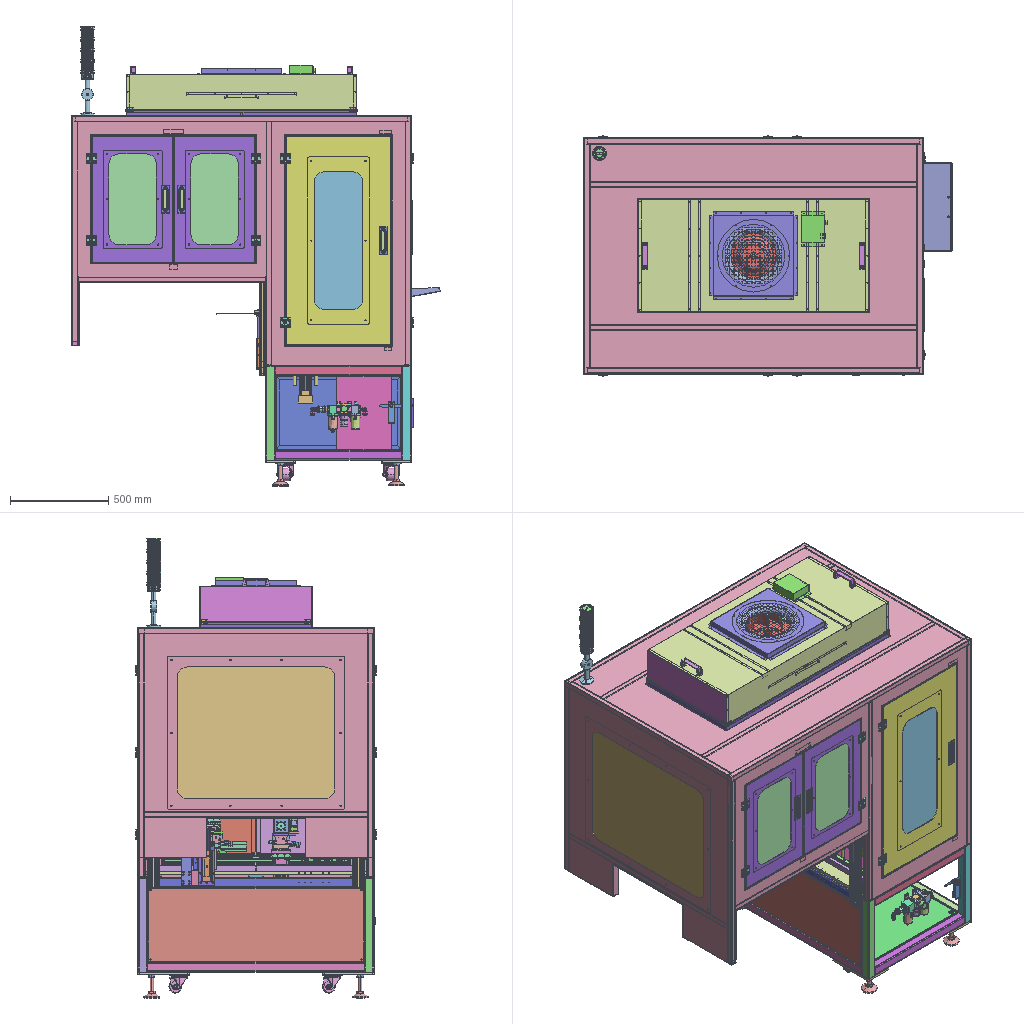Assembly | SolidWorks | 289 different items | 600 placed | box 1872 x 1223 x 2337 mm
Parts list (item | name | quantity | parent item | size | volume | features):
1 | (subassembly) | x1 | in 13 | 206.7 x 78.5 x 62 mm | 306344 mm3 | -
2 | (subassembly) | x1 | in 1 | 184.2 x 78.5 x 62 mm | 299098 mm3 | -
3 | (subassembly) | x1 | in 4 | 25 x 39 x 62 mm | 38108 mm3 | -
4 | (subassembly) | x1 | in 5 | 25 x 39 x 62 mm | 38108 mm3 | -
5 | (subassembly) | x1 | in 6 | 25 x 39 x 62 mm | 38108 mm3 | -
6 | (subassembly) | x1 | in 2 | 184.2 x 78.5 x 62 mm | 299098 mm3 | -
7 | (subassembly) | x1 | in 3 | 25 x 39 x 62 mm | 38108 mm3 | -
8 | (subassembly) | x1 | in 9 | 1174 x 574 x 303.9 mm | 75861290 mm3 | -
9 | (subassembly) | x1 | - | - | - | features InContextFeatHolder 8, CompositeCurve 1
10 | (subassembly) | x1 | in 12 | 740 x 1200 x 627 mm | 11363553 mm3 | features InContextFeatHolder 2
11 | (subassembly) | x1 | in 13 | 74.6 x 107 x 490 mm | 263242 mm3 | -
12 | (subassembly) | x1 | in 9 | - | 46022542 mm3 | features InContextFeatHolder 11, CompositeCurve 1
13 | (subassembly) | x1 | - | - | - | features InContextFeatHolder 122, ReferencePattern 9, AEMSimFeature 1, LocalLPattern 1
14 | (subassembly) | x1 | - | - | 2657898 mm3 | features InContextFeatHolder 6
15 | (subassembly) | x1 | in 13 | 960 x 40 x 48 mm | 597195 mm3 | -
16 | (subassembly) | x2 | in 13 | 570.077 x 115 x 65.1 mm | 63458 mm3 | features AEMSimFeature 1
17 | (subassembly) | x3 | in 13 | 380 x 48 x 106.85 mm | 542226 mm3 | -
18 | (subassembly) | x1 | in 27 | 150 x 20.749 x 140 mm | 48945 mm3 | -
19 | (subassembly) | x2 | in 13 | 60 x 10 x 20 mm | 6249 mm3 | -
20 | (subassembly) | x1 | in 13 | 80 x 32 x 65 mm | 107710 mm3 | features AEMSimFeature 1
21 | (subassembly) | x1 | in 13 | 97.6 x 32 x 65 mm | 120798 mm3 | features AEMSimFeature 1
22 | (subassembly) | x1 | in 31 | 62 x 9.5 x 27.6 mm | 10978 mm3 | -
23 | (subassembly) | x2 | in 13 | 175.3 x 32 x 65 mm | 205284 mm3 | features AEMSimFeature 1
24 | (subassembly) | x1 | in 13 | - | 4425715 mm3 | -
25 | (subassembly) | x2 | in 13 | 342 x 153.7 x 73.7 mm | 1636225 mm3 | -
26 | (subassembly) | x2 | in 24 | 88.4 x 8 x 103.5 mm | 9214 mm3 | -
27 | (subassembly) | x1 | in 9 | - | 566898 mm3 | -
28 | (subassembly) | x1 | in 14 | 204 x 189.5 x 238.5 mm | 703378 mm3 | -
29 | (subassembly) | x16 | in 12 | 50 x 11.3 x 50 mm | 15084 mm3 | -
30 | (subassembly) | x1 | in 22 | 62 x 9.5 x 27.6 mm | 10978 mm3 | -
31 | (subassembly) | x1 | in 7 | 25 x 39 x 62 mm | 38108 mm3 | -
32 | (subassembly) | x1 | in 27 | 244 x 14 x 167 mm | 40876 mm3 | -
33 | (subassembly) | x1 | in 9 | 167.4 x 157.9 x 105 mm | 781084 mm3 | features AEMSimFeature 1
34 | (subassembly) | x4 | in 10 | 185 x 80 x 80 mm | 147831 mm3 | -
35 | (subassembly) | x1 | in 13 | 179 x 58 x 20 mm | 151640 mm3 | features AEMSimFeature 1
36 | - | x2 | in 1 | 20 x 10 x 27.5 mm | 2836 mm3 | features BaseBody 1
37 | - | x2 | in 13 | 84 x 700 x 12 mm | 143164 mm3 | features HoleWzd 3, Fillet 1, FlatPattern 1, SMBaseFlange 1, SheetMetal 1
38 | - | x1 | in 13 | 70 x 25 x 57 mm | 49488 mm3 | features HoleWzd 2, Chamfer 1, Extrusion 1, ICE 1
39 | - | x4 | in 13 | 65 x 11 x 12 mm | 4036 mm3 | features ICE 5, Chamfer 4, Fillet 2, Extrusion 1, HoleWzd 1
40 | - | x1 | in 13 | 78 x 80 x 108.5 mm | 46050 mm3 | features HoleWzd 2, Fillet 1, FlatPattern 1, SMBaseFlange 1, SheetMetal 1
41 | - | x1 | in 13 | 120 x 20 x 10 mm | 22814 mm3 | features HoleWzd 2, ICE 2, Chamfer 1, Extrusion 1, LPattern 1
42 | - | x1 | in 13 | 80 x 15 x 180 mm | 211462 mm3 | features HoleWzd 3, Chamfer 1, Extrusion 1
43 | - | x1 | in 13 | 60 x 10 x 50 mm | 26983 mm3 | features HoleWzd 3, Chamfer 1, Extrusion 1, ICE 1
44 | - | x2 | in 13 | 50 x 8 x 56 mm | 20280 mm3 | features HoleWzd 8, Chamfer 2, Extrusion 1
45 | - | x1 | in 13 | 46.5 x 10 x 50 mm | 20990 mm3 | features HoleWzd 2, Chamfer 1, Extrusion 1
46 | - | x1 | in 13 | 25 x 10 x 110 mm | 24285 mm3 | features HoleWzd 3, Chamfer 1, Extrusion 1, ICE 1
47 | - | x1 | in 30 | 62 x 27.6 x 9.5 mm | 10978 mm3 | features BaseBody 1
48 | - | x1 | in 13 | 143 x 40 x 32 mm | 20017 mm3 | features HoleWzd 2, Fillet 1, FlatPattern 1, SMBaseFlange 1, SheetMetal 1
49 | - | x1 | in 13 | 233 x 40 x 32 mm | 34041 mm3 | features HoleWzd 2, ICE 2, Fillet 1, FlatPattern 1, SMBaseFlange 1, SheetMetal 1
50 | - | x1 | in 13 | 200 x 10 x 50 mm | 97100 mm3 | features HoleWzd 5, Chamfer 1, Extrusion 1
51 | - | x1 | in 13 | 50 x 10 x 240 mm | 114088 mm3 | features HoleWzd 2, Chamfer 1, Extrusion 1
52 | - | x1 | in 13 | 60 x 35 x 25.5 mm | 8094 mm3 | features HoleWzd 2, Fillet 1, FlatPattern 1, SMBaseFlange 1, SheetMetal 1
53 | - | x1 | in 13 | 80 x 40 x 75 mm | 17875 mm3 | features HoleWzd 2, Fillet 1, FlatPattern 1, SMBaseFlange 1, SheetMetal 1
54 | - | x1 | in 13 | 100 x 30 x 53 mm | 13622 mm3 | features HoleWzd 2, Fillet 1, FlatPattern 1, ICE 1, SMBaseFlange 1, SheetMetal 1
55 | - | x1 | in 13 | 70 x 50 x 75 mm | 19314 mm3 | features Fillet 2, HoleWzd 2, FlatPattern 1, ICE 1, SMBaseFlange 1, SheetMetal 1
56 | - | x2 | in 13 | 50 x 65 x 50.5 mm | 18737 mm3 | features HoleWzd 2, Fillet 1, FlatPattern 1, ICE 1, SMBaseFlange 1, SheetMetal 1
57 | - | x1 | in 13 | 70 x 50 x 75 mm | 19314 mm3 | features Fillet 2, HoleWzd 2, FlatPattern 1, ICE 1, SMBaseFlange 1, SheetMetal 1
58 | - | x1 | in 18 | 7.55 x 3.6 x 5.25 mm | 54.106 mm3 | features BaseBody 5
59 | - | x1 | in 13 | 170 x 10 x 75 mm | 122534 mm3 | features Chamfer 1, Cut 1, Extrusion 1
60 | - | x1 | in 13 | 67 x 70.75 x 50 mm | 14918 mm3 | features ICE 4, EdgeFlange 2, FlatPattern 2, HoleWzd 2, SMBaseFlange 2, SheetMetal 2, Fillet 1
61 | - | x1 | in 13 | 90 x 5 x 60 mm | 26435 mm3 | features Chamfer 1, Cut 1, Extrusion 1
62 | - | x1 | in 13 | 67 x 90.75 x 50 mm | 17594 mm3 | features ICE 5, EdgeFlange 2, Fillet 2, FlatPattern 2, HoleWzd 2, SMBaseFlange 2, SheetMetal 2, MirrorSolid 1
63 | - | x1 | in 13 | 27 x 70 x 27 mm | 8082 mm3 | features HoleWzd 2, EdgeFlange 1, Fillet 1, FlatPattern 1, ICE 1, SMBaseFlange 1, SheetMetal 1
64 | - | x1 | - | 27 x 70 x 27 mm | 8082 mm3 | features HoleWzd 2, ICE 2, EdgeFlange 1, Fillet 1, FlatPattern 1, MirrorSolid 1, SMBaseFlange 1, SheetMetal 1
65 | - | x2 | in 13 | 100 x 30 x 60 mm | 72680 mm3 | features HoleWzd 2, Chamfer 1, Extrusion 1, ICE 1
66 | - | x1 | in 13 | 65 x 46.5 x 55 mm | 13185 mm3 | features HoleWzd 4, ICE 3, EdgeFlange 2, FlatPattern 2, SMBaseFlange 2, SheetMetal 2, Cut 1, Fillet 1
67 | - | x1 | in 13 | 65 x 31.5 x 55 mm | 13652 mm3 | features HoleWzd 4, EdgeFlange 2, FlatPattern 2, ICE 2, SMBaseFlange 2, SheetMetal 2, Fillet 1
68 | - | x1 | in 13 | 50 x 3 x 45 mm | 6177 mm3 | features Chamfer 1, Extrusion 1, HoleWzd 1
69 | - | x1 | in 18 | 5.1 x 2 x 11 mm | 74.432 mm3 | features BaseBody 1
70 | - | x2 | in 13 | 30 x 22 x 30 mm | 5974 mm3 | features HoleWzd 3, ICE 2, Chamfer 1, Extrusion 1
71 | - | x2 | in 13 | 25 x 30 x 60 mm | 17122 mm3 | features HoleWzd 3, ICE 2, Chamfer 1, Extrusion 1
72 | - | x2 | in 13 | 8 x 75 x 8 mm | 3681 mm3 | features Extrusion 1, HoleWzd 1
73 | - | x2 | in 13 | 10 x 25 x 20 mm | 4403 mm3 | features HoleWzd 3, Chamfer 1, Extrusion 1, ICE 1
74 | - | x2 | in 13 | 12 x 15 x 20 mm | 2799 mm3 | features Chamfer 1, Extrusion 1, HoleWzd 1
75 | - | x2 | in 14 | 30 x 60 x 560 mm | 279456 mm3 | features HoleWzd 1, WeldMemberFeat 1, WeldmentFeature 1
76 | - | x1 | in 14 | 30 x 60 x 980 mm | 490298 mm3 | features WeldMemberFeat 1, WeldmentFeature 1
77 | - | x2 | in 14 | 63 x 60 x 63 mm | 21324 mm3 | features HoleWzd 2, Fillet 1, FlatPattern 1, ICE 1, SMBaseFlange 1, SheetMetal 1
78 | - | x1 | - | 30 x 60 x 300 mm | 150091 mm3 | features WeldMemberFeat 1, WeldmentFeature 1
79 | - | x1 | - | 60 x 60 x 60 mm | 62996 mm3 | features HoleWzd 2, Chamfer 1, Extrusion 1, ICE 1
80 | - | x1 | in 18 | 28.83 x 2.1 x 4.91 mm | 297.266 mm3 | features BaseBody 1
81 | - | x2 | in 14 | 120 x 10 x 120 mm | 98760 mm3 | features Chamfer 1, Extrusion 1, Fillet 1, HoleWzd 1, ICE 1
82 | - | x1 | in 14 | 230 x 10 x 205 mm | 459180 mm3 | features HoleWzd 3, Chamfer 1, Extrusion 1
83 | - | x2 | in 14 | 120 x 10 x 60 mm | 66873 mm3 | features HoleWzd 3, Chamfer 1, Extrusion 1
84 | - | x2 | in 14 | 90 x 10 x 60 mm | 36102 mm3 | features HoleWzd 2, Chamfer 1, Extrusion 1, ICE 1
85 | - | x4 | in 12 | 414.5 x 646 x 20 mm | 455877 mm3 | features HoleWzd 3, ICE 3, EdgeFlange 2, Cut 1, FlatPattern 1, LPattern 1, SMBaseFlange 1, SheetMetal 1
86 | - | x4 | in 12 | 300 x 500 x 5 mm | 748723 mm3 | features Extrusion 1, Fillet 1, HoleWzd 1
87 | - | x1 | in 27 | 235 x 5 x 143 mm | 168025 mm3 | features BaseBody 1
88 | - | x1 | in 33 | 37.5 x 37.5 x 40.6 mm | 27619 mm3 | features BaseBody 1
89 | - | x1 | in 15 | 48 x 34.5 x 84 mm | 102162 mm3 | features BaseBody 5
90 | - | x1 | in 15 | 48 x 34.5 x 84 mm | 102161 mm3 | features BaseBody 5
91 | - | x1 | in 18 | 16 x 8.47 x 16.6 mm | 886.614 mm3 | features BaseBody 1
92 | - | x1 | in 15 | 23 x 22 x 960 mm | 392872 mm3 | features BaseBody 1
93 | - | x1 | in 13 | 32 x 55 x 30 mm | 32416 mm3 | features ICE 2, Extrusion 1, HoleWzd 1, LPattern 1
94 | - | x1 | in 13 | - | - | features BaseBody 3, RefSurface 1
95 | - | x8 | in 9 | 30 x 91 x 31 mm | 76497 mm3 | features BaseBody 2
96 | - | x8 | in 9 | 48.4 x 47.5 x 16.6 mm | 8438 mm3 | features BaseBody 7, MoveCopyBody 1
97 | - | x1 | in 9 | 35.5 x 35.5 x 68.5 mm | 34572 mm3 | features BaseBody 2
98 | - | x1 | in 18 | 47.6 x 49.1 x 3.35 mm | 7804 mm3 | features BaseBody 1
99 | - | x3 | in 13 | 174.25 x 62 x 80 mm | 431030 mm3 | features HoleWzd 2, Sweep 1
100 | - | x4 | in 16 | 32 x 7 x 58 mm | 8749 mm3 | features BaseBody 1
101 | - | x2 | in 16 | 58.5 x 35 x 65 mm | 23683 mm3 | features BaseBody 1
102 | - | x1 | in 18 | 14.571 x 11.26 x 19.95 mm | 1672 mm3 | features BaseBody 1
103 | - | x2 | in 16 | 58.5 x 35 x 65 mm | 22276 mm3 | features BaseBody 1
104 | - | x30 | in 16 | - | - | features BaseBody 1
105 | - | x3 | in 17 | 94 x 36 x 82.5 mm | 126431 mm3 | features BaseBody 1
106 | - | x3 | in 17 | 62 x 47 x 370 mm | 387917 mm3 | features BaseBody 1
107 | - | x3 | in 17 | 42 x 42 x 11 mm | 10971 mm3 | features BaseBody 1
108 | - | x3 | in 17 | 8 x 5 x 300 mm | 5669 mm3 | features BaseBody 1
109 | - | x6 | in 17 | 27.675 x 17 x 32.6 mm | 3746 mm3 | features BaseBody 1
110 | - | x3 | in 17 | 27.675 x 17 x 32.6 mm | 3746 mm3 | features BaseBody 1
111 | - | x8 | in 13 | 34 x 48 x 70 mm | 33372 mm3 | features BaseBody 1
112 | - | x2 | in 13 | 24 x 32 x 21 mm | 5040 mm3 | features HoleWzd 2, ICE 2, CirPattern 1, Extrusion 1
113 | - | x1 | in 18 | 15.807 x 7.64 x 18.249 mm | 686.202 mm3 | features BaseBody 1
114 | - | x8 | in 12 | - | - | features BaseBody 6, RefSurface 2
115 | - | x8 | in 12 | 13 x 13 x 37 mm | 2260 mm3 | features ICE 2, Extrusion 1
116 | - | x2 | in 19 | 20 x 8 x 28.9 mm | 3330 mm3 | features BaseBody 5
117 | - | x2 | in 19 | 9 x 6.5 x 60 mm | 2919 mm3 | features BaseBody 1, ICE 1
118 | - | x3 | in 12 | 120 x 110 x 37 mm | 69257 mm3 | features ICE 6, Fillet 4, Chamfer 1, Extrusion 1, MirrorPattern 1
119 | - | x1 | in 18 | 150 x 1.6 x 140 mm | 32858 mm3 | features BaseBody 1
120 | - | x1 | in 20 | 8 x 8 x 20 mm | 908.839 mm3 | features BaseBody 1
121 | - | x1 | in 21 | 8 x 8 x 20 mm | 908.839 mm3 | features BaseBody 1
122 | - | x1 | in 20 | 12 x 13.856 x 4 mm | 340.073 mm3 | features BaseBody 1
123 | - | x1 | in 21 | 12 x 13.856 x 4 mm | 340.073 mm3 | features BaseBody 1
124 | - | x1 | in 18 | 18.3 x 13.55 x 20.425 mm | 1911 mm3 | features BaseBody 1
125 | - | x1 | in 20 | 13 x 10 x 18.5 mm | 2290 mm3 | features BaseBody 1
126 | - | x1 | in 21 | 13 x 10 x 18.5 mm | 2290 mm3 | features BaseBody 1
127 | - | x1 | in 20 | 16 x 31 x 9.5 mm | 4071 mm3 | features BaseBody 1
128 | - | x1 | in 21 | 16 x 31 x 9.5 mm | 4071 mm3 | features BaseBody 1
129 | - | x2 | in 23 | 12 x 13.856 x 4 mm | 339.344 mm3 | features BaseBody 1
130 | - | x2 | in 23 | 16 x 31 x 9.5 mm | 4071 mm3 | features BaseBody 1
131 | - | x2 | in 23 | 15 x 10 x 20.5 mm | 2936 mm3 | features BaseBody 1
132 | - | x1 | in 20 | 47 x 26.5 x 70 mm | 54767 mm3 | features BaseBody 1
133 | - | x1 | in 20 | 50 x 29 x 79 mm | 45333 mm3 | features BaseBody 1
134 | - | x1 | in 21 | 47 x 26.5 x 82 mm | 60945 mm3 | features BaseBody 1
135 | - | x1 | in 18 | 12.55 x 30.81 x 17.2 mm | 2595 mm3 | features BaseBody 1
136 | - | x1 | in 21 | 50 x 29 x 91 mm | 51453 mm3 | features BaseBody 1
137 | - | x2 | in 23 | 47 x 26.5 x 148 mm | 111370 mm3 | features BaseBody 1
138 | - | x2 | in 23 | 50 x 29 x 157 mm | 83904 mm3 | features BaseBody 1
139 | - | x4 | in 23 | 4 x 4.5 x 32 mm | 371.041 mm3 | features BaseBody 1
140 | - | x2 | in 21 | 4 x 4.6 x 32 mm | 394.901 mm3 | features BaseBody 1
141 | - | x2 | in 9 | 39.315 x 43.5 x 21 mm | 8972 mm3 | features BaseBody 1
142 | - | x1 | in 1 | 26 x 14.6 x 15 mm | 1573 mm3 | features BaseBody 1
143 | - | x1 | in 9 | 70.234 x 70.234 x 455.4 mm | 394437 mm3 | features BaseBody 7, ICE 3, HoleWzd 2, MoveCopyBody 2, Fillet 1, Stock 1
144 | - | x2 | in 23 | 40.8 x 8 x 8 mm | 1922 mm3 | features BaseBody 1
145 | - | x1 | in 24 | 111.5 x 65 x 930 mm | 2439001 mm3 | features BaseBody 1
146 | - | x2 | in 25 | 66 x 153.7 x 73.7 mm | 524203 mm3 | features BaseBody 1
147 | - | x1 | in 18 | 7.5 x 10.5 x 3.3 mm | 105.725 mm3 | features BaseBody 1
148 | - | x2 | in 24 | 110 x 49 x 100 mm | 206200 mm3 | features BaseBody 1
149 | - | x1 | in 24 | 82 x 17.089 x 949 mm | 309530 mm3 | features BaseBody 1
150 | - | x2 | in 24 | 920 x 12.53 x 15 mm | 149023 mm3 | features BaseBody 1
151 | - | x8 | in 24 | 40.3 x 19.5 x 34 mm | 21226 mm3 | features BaseBody 1
152 | - | x2 | in 9 | 120 x 120 x 25 mm | 99576 mm3 | features Boss 5, Fillet 2, CirPattern 1, Cut 1, Extrusion 1, HoleWzd 1
153 | - | x2 | in 25 | 60 x 171.6 x 72.85 mm | 479622 mm3 | features BaseBody 1
154 | - | x1 | - | 51 x 26 x 73 mm | 95067 mm3 | features Extrusion 1, Fillet 1, HoleWzd 1, ICE 1
155 | - | x2 | in 13 | 5 x 15 x 5 mm | 252.815 mm3 | features Chamfer 1, Extrusion 1, HoleWzd 1
156 | - | x2 | in 33 | 16.2 x 43 x 13.5 mm | 6701 mm3 | features BaseBody 1
157 | - | x2 | in 33 | 7.5 x 43 x 30 mm | 4813 mm3 | features BaseBody 1
158 | - | x12 | in 27 | 6 x 10 x 6 mm | 109.62 mm3 | features BaseBody 1
159 | - | x2 | in 33 | 20 x 85 x 28 mm | 22186 mm3 | features BaseBody 1
160 | - | x2 | in 26 | 31 x 8 x 25 mm | 3494 mm3 | features BaseBody 1
161 | - | x2 | in 26 | 76.4 x 83.5 x 7 mm | 5719 mm3 | features BaseBody 1
162 | - | x2 | in 24 | 50 x 53.1 x 100 mm | 115973 mm3 | features BaseBody 1
163 | - | x2 | in 24 | 18 x 18 x 1.5 mm | 454.137 mm3 | features BaseBody 1
164 | - | x1 | in 24 | 50 x 10.1 x 120 mm | 50542 mm3 | features BaseBody 1
165 | - | x4 | in 24 | 50 x 10.1 x 200 mm | 84250 mm3 | features BaseBody 1
166 | - | x2 | in 24 | 18 x 14 x 4 mm | 787.982 mm3 | features BaseBody 1
167 | - | x2 | in 24 | 45 x 15 x 17 mm | 8178 mm3 | features BaseBody 1
168 | - | x2 | in 24 | 56.42 x 14.8 x 12 mm | 6251 mm3 | features BaseBody 1
169 | - | x1 | in 27 | 265 x 193 x 0.32 mm | 7343 mm3 | features BaseBody 1
170 | - | x4 | in 24 | 17 x 17 x 10 mm | 1547 mm3 | features BaseBody 1
171 | - | x1 | in 13 | 158.45 x 26.5 x 60 mm | 118461 mm3 | features BaseBody 3
172 | - | x2 | in 8 | 19.9 x 568.8 x 179.4 mm | 76913 mm3 | features BaseBody 1
173 | - | x2 | in 8 | 58.8 x 560 x 25 mm | 35807 mm3 | features BaseBody 1
174 | - | x1 | in 28 | 11 x 38.188 x 38.188 mm | 8381 mm3 | features BaseBody 1
175 | - | x1 | - | 27 x 11 x 89 mm | 6132 mm3 | features ICE 3, Chamfer 2, Fillet 2, ExtruThin 1
176 | - | x1 | in 8 | 29.6 x 34.2 x 22.3 mm | 11730 mm3 | features BaseBody 1
177 | - | x2 | in 8 | 136.5 x 40 x 26 mm | 27538 mm3 | features BaseBody 1
178 | - | x1 | - | 27 x 11 x 89 mm | 6132 mm3 | features Fillet 2, ICE 2, Chamfer 1, ExtruThin 1
179 | - | x1 | in 28 | 203 x 228 x 6 mm | 252836 mm3 | features BaseBody 1
180 | - | x2 | in 32 | 10 x 2 x 21 mm | 420 mm3 | features BaseBody 1
181 | - | x1 | in 8 | 178.6 x 44.9 x 114.8 mm | 25020 mm3 | features BaseBody 1
182 | - | x1 | in 28 | 110 x 40 x 10 mm | 12474 mm3 | features BaseBody 1
183 | - | x1 | in 9 | 270 x 35 x 167 mm | 892435 mm3 | features Fillet 3, ICE 3, Extrusion 1, HoleWzd 1
184 | - | x11 | in 13 | 2 x 34 x 2 mm | 106.814 mm3 | features Extrusion 1
185 | - | x1 | in 8 | 40 x 20 x 40 mm | 945.968 mm3 | features BaseBody 1
186 | - | x1 | in 8 | 170 x 568.8 x 20 mm | 69593 mm3 | features BaseBody 1
187 | - | x1 | in 28 | 58 x 13.5 x 49 mm | 21022 mm3 | features BaseBody 1
188 | - | x1 | in 28 | 203 x 133.5 x 222.9 mm | 123342 mm3 | features BaseBody 1
189 | - | x1 | in 8 | 1169 x 570 x 180 mm | 606575 mm3 | features BaseBody 1
190 | - | x1 | in 8 | 560 x 568.8 x 17.4 mm | 168286 mm3 | features BaseBody 1
191 | - | x1 | in 27 | 270.8 x 5.7 x 198.8 mm | 17493 mm3 | features BaseBody 1
192 | - | x1 | in 28 | 13 x 35 x 35 mm | 3307 mm3 | features BaseBody 1
193 | - | x1 | in 28 | 204 x 141.5 x 3.5 mm | 90063 mm3 | features BaseBody 1
194 | - | x4 | in 28 | 19.046 x 16 x 19.046 mm | 2136 mm3 | features BaseBody 1
195 | - | x4 | in 11 | 19.513 x 16 x 19.513 mm | 2386 mm3 | features BaseBody 1
196 | - | x1 | in 8 | 30 x 30 x 37 mm | 14720 mm3 | features BaseBody 1
197 | - | x3 | in 11 | 5 x 8 x 8 mm | 228.346 mm3 | features BaseBody 1
198 | - | x2 | in 8 | 40 x 20 x 40 mm | 945.968 mm3 | features BaseBody 1
199 | - | x1 | in 8 | 40 x 20 x 40 mm | 945.968 mm3 | features BaseBody 1
200 | - | x1 | in 13 | 36 x 28.1 x 36 mm | 26906 mm3 | features Extrusion 1, ICE 1
201 | - | x1 | in 11 | 347 x 40 x 40 mm | 65836 mm3 | features BaseBody 1, ICE 1
202 | - | x1 | in 27 | 35.585 x 17.1 x 141.528 mm | 13223 mm3 | features BaseBody 1
203 | - | x1 | - | 8 x 8 x 20 mm | 605.018 mm3 | features Chamfer 1, Extrusion 1, ICE 1, MirrorPattern 1
204 | - | x1 | in 28 | 222.8 x 84 x 5 mm | 93378 mm3 | features BaseBody 1
205 | - | x1 | in 28 | 204 x 141.5 x 3.5 mm | 90078 mm3 | features BaseBody 1
206 | - | x2 | in 9 | 117.5 x 5.2 x 117.5 mm | 4285 mm3 | features Boss 1, CompositeCurve 1, MirrorPattern 1, Revolution 1, Sweep 1
207 | - | x1 | in 8 | 1170 x 79 x 570 mm | 72868307 mm3 | features BaseBody 6
208 | - | x1 | in 27 | 272.622 x 33.34 x 200.622 mm | 144122 mm3 | features BaseBody 1
209 | - | x1 | in 27 | 256 x 1 x 184 mm | 42983 mm3 | features BaseBody 1
210 | - | x1 | in 32 | 244 x 12 x 167 mm | 40036 mm3 | features BaseBody 1
211 | - | x1 | in 8 | 395 x 93 x 395 mm | 708479 mm3 | features BaseBody 1
212 | - | x2 | in 25 | 200 x 53 x 53 mm | 525174 mm3 | features BaseBody 1
213 | - | x1 | in 8 | 370 x 30.2 x 370 mm | 96881 mm3 | features BaseBody 1
214 | - | x1 | in 8 | 154 x 120 x 154 mm | 897140 mm3 | features BaseBody 2
215 | - | x1 | in 8 | 448.8 x 29.9 x 448.6 mm | 111813 mm3 | features BaseBody 1
216 | - | x2 | in 24 | 22 x 37.5 x 8 mm | 1327 mm3 | features BaseBody 1
217 | - | x1 | in 27 | 152.5 x 244.9 x 2.34 mm | 82614 mm3 | features BaseBody 1
218 | - | x1 | in 31 | 54 x 39 x 15.5 mm | 27130 mm3 | features BaseBody 1
219 | - | x1 | in 33 | 53 x 53.5 x 53 mm | 128683 mm3 | features BaseBody 1
220 | - | x1 | in 33 | 46.4 x 74.3 x 53.2 mm | 114599 mm3 | features BaseBody 1
221 | - | x1 | in 33 | 19.5 x 11.1 x 8 mm | 1041 mm3 | features BaseBody 1
222 | - | x1 | in 33 | 53 x 70.1 x 53 mm | 131657 mm3 | features BaseBody 1
223 | - | x2 | in 24 | 110 x 15 x 92 mm | 55640 mm3 | features BaseBody 1
224 | - | x1 | in 33 | 46.4 x 74.3 x 53.2 mm | 114523 mm3 | features BaseBody 1
225 | - | x1 | in 33 | 53 x 52 x 53 mm | 114626 mm3 | features BaseBody 1
226 | - | x1 | in 33 | 53 x 65 x 53 mm | 80542 mm3 | features BaseBody 1
227 | - | x4 | in 34 | 185 x 80 x 80 mm | 139335 mm3 | features BaseBody 1
228 | - | x4 | in 34 | 16 x 34.641 x 30 mm | 8496 mm3 | features BaseBody 1
229 | - | x4 | in 10 | 102.5 x 95 x 100 mm | 269431 mm3 | features BaseBody 4
230 | - | x32 | in 29 | 31 x 11.3 x 50 mm | 6837 mm3 | features BaseBody 1
231 | - | x16 | in 29 | 6 x 6 x 50 mm | 1409 mm3 | features MoveCopyBody 5, BaseBody 1
232 | - | x1 | in 35 | 20 x 58 x 169 mm | 126513 mm3 | features BaseBody 1
233 | - | x1 | in 35 | 18 x 56 x 154 mm | 25127 mm3 | features BaseBody 1
234 | - | x1 | in 33 | 9.728 x 9.728 x 6.2 mm | 395.486 mm3 | features BaseBody 1
235 | - | x1 | in 6 | 160.8 x 46.8 x 78.5 mm | 260990 mm3 | features BaseBody 1
236 | - | x1 | - | 33 x 37.5 x 33 mm | 22047 mm3 | features Chamfer 1, Extrusion 1, RevCut 1
237 | - | x1 | - | 40 x 40 x 39 mm | 38929 mm3 | features Extrusion 1, ICE 1
238 | - | x2 | in 9 | 148.5 x 148.5 x 29 mm | 366901 mm3 | features HoleWzd 2, ICE 2, Extrusion 1, LPattern 1
239 | - | x3 | in 13 | 117.111 x 104.2 x 58.651 mm | 144018 mm3 | features BaseBody 2
240 | - | x4 | in 24 | 13.7 x 28.4 x 26 mm | 1939 mm3 | features BaseBody 1
241 | - | x1 | in 10 | 50 x 50 x 480 mm | 259595 mm3 | features WeldMemberFeat 1, WeldmentFeature 1
242 | - | x1 | in 10 | 50 x 50 x 480 mm | 259595 mm3 | features WeldMemberFeat 1, WeldmentFeature 1
243 | - | x1 | in 10 | 50 x 50 x 640 mm | 345950 mm3 | features HoleWzd 1, WeldMemberFeat 1, WeldmentFeature 1
244 | - | x1 | in 10 | 50 x 50 x 640 mm | 346127 mm3 | features WeldMemberFeat 1, WeldmentFeature 1
245 | - | x1 | in 11 | 170 x 73 x 8 mm | 75730 mm3 | features BaseBody 1
246 | - | x1 | in 10 | 50 x 50 x 1100 mm | 594670 mm3 | features HoleWzd 1, WeldMemberFeat 1, WeldmentFeature 1
247 | - | x1 | in 10 | 50 x 50 x 640 mm | 346127 mm3 | features WeldMemberFeat 1, WeldmentFeature 1
248 | - | x1 | in 10 | 50 x 50 x 640 mm | 345950 mm3 | features HoleWzd 1, WeldMemberFeat 1, WeldmentFeature 1
249 | - | x1 | in 10 | 50 x 50 x 480 mm | 259595 mm3 | features WeldMemberFeat 1, WeldmentFeature 1
250 | - | x1 | in 10 | 50 x 50 x 1100 mm | 594018 mm3 | features HoleWzd 4, WeldMemberFeat 1, WeldmentFeature 1
251 | - | x1 | in 10 | 50 x 50 x 1100 mm | 594905 mm3 | features WeldMemberFeat 1, WeldmentFeature 1
252 | - | x1 | in 10 | 50 x 50 x 1100 mm | 594905 mm3 | features WeldMemberFeat 1, WeldmentFeature 1
253 | - | x1 | in 10 | 50 x 50 x 480 mm | 259595 mm3 | features WeldMemberFeat 1, WeldmentFeature 1
254 | - | x4 | in 10 | 150 x 12 x 260 mm | 462019 mm3 | features HoleWzd 2, Extrusion 1, Fillet 1
255 | - | x4 | in 10 | 44 x 3 x 44 mm | 5785 mm3 | features Extrusion 1, Fillet 1
256 | - | x1 | in 11 | 73.2 x 90 x 163.5 mm | 60174 mm3 | features BaseBody 1
257 | - | x1 | in 10 | 20 x 1100 x 640 mm | 1523319 mm3 | features Cut 1, EdgeFlange 1, FlatPattern 1, SMBaseFlange 1, SheetMetal 1
258 | - | x4 | in 10 | 40 x 5 x 40 mm | 3902 mm3 | features Extrusion 1, HoleWzd 1
259 | - | x9 | in 10 | 80 x 15 x 80 mm | 95133 mm3 | features Extrusion 1, Fillet 1, HoleWzd 1
260 | - | x1 | in 10 | 50 x 50 x 1100 mm | 594905 mm3 | features WeldMemberFeat 1, WeldmentFeature 1
261 | - | x3 | in 10 | 45 x 10 x 40 mm | 11000 mm3 | features Extrusion 1, ICE 1
262 | - | x1 | in 12 | 560 x 402 x 22 mm | 485747 mm3 | features MoveCopyBody 4, Stock 4, EdgeFlange 3, ICE 2, Cut 1, FlatPattern 1, LPattern 1, SMBaseFlange 1, SheetMetal 1
263 | - | x1 | in 12 | 376 x 1096 x 20 mm | 1022665 mm3 | features EdgeFlange 2, FlatPattern 1, HoleWzd 1, SMBaseFlange 1, SheetMetal 1
264 | - | x1 | in 12 | 636 x 390 x 20 mm | 609250 mm3 | features EdgeFlange 2, MoveCopyBody 2, Stock 2, FlatPattern 1, ICE 1, SMBaseFlange 1, SheetMetal 1
265 | - | x1 | in 12 | 1270 x 1200 x 1725 mm | 14201565 mm3 | features EdgeFlange 19, ICE 17, FlatPattern 11, HoleWzd 11, Fillet 7, SMBaseFlange 7, SheetMetal 7, MirrorSolid 2, 3DProfileFeature 1, Cut 1, MirrorPattern 1, WeldMemberFeat 1, WeldmentFeature 1
266 | - | x2 | in 12 | 315 x 850 x 5 mm | 1337473 mm3 | features Extrusion 1, Fillet 1, HoleWzd 1
267 | - | x1 | in 11 | 74 x 98 x 4.5 mm | 27198 mm3 | features BaseBody 1
268 | - | x2 | in 12 | 536 x 1066 x 20 mm | 1021642 mm3 | features ICE 4, HoleWzd 3, EdgeFlange 2, Cut 1, FlatPattern 1, LPattern 1, SMBaseFlange 1, SheetMetal 1
269 | - | x1 | in 12 | 497 x 1066 x 20 mm | 1161554 mm3 | features Cut 2, EdgeFlange 2, HoleWzd 2, ICE 2, LPattern 2, FlatPattern 1, SMBaseFlange 1, SheetMetal 1
270 | - | x1 | in 12 | 497 x 1066 x 48 mm | 1342726 mm3 | features Cut 6, EdgeFlange 4, HoleWzd 4, FlatPattern 2, SMBaseFlange 2, SheetMetal 2, ICE 1
271 | - | x1 | in 12 | 448 x 165 x 40 mm | 228606 mm3 | features ICE 4, EdgeFlange 3, HoleWzd 3, Fillet 1, FlatPattern 1, SMBaseFlange 1, SheetMetal 1
272 | - | x1 | in 12 | 40 x 41.5 x 80 mm | 9432 mm3 | features Fillet 1, FlatPattern 1, HoleWzd 1, SMBaseFlange 1, SheetMetal 1
273 | - | x1 | in 12 | 280 x 550 x 375 mm | 1500935 mm3 | features EdgeFlange 3, Cut 2, ICE 2, FlatPattern 1, SMBaseFlange 1, SheetMetal 1
274 | - | x1 | in 12 | 15 x 325 x 500 mm | 418730 mm3 | features EdgeFlange 2, FlatPattern 1, ICE 1, SMBaseFlange 1, SheetMetal 1
275 | - | x1 | in 12 | 900 x 780 x 5 mm | 3507647 mm3 | features Extrusion 1, Fillet 1, HoleWzd 1
276 | - | x1 | in 13 | 1120 x 15 x 700 mm | 9247441 mm3 | features HoleWzd 10, Cut 2, Chamfer 1, Extrusion 1, Fillet 1
277 | - | x1 | in 13 | 100 x 15 x 350 mm | 438251 mm3 | features HoleWzd 6, ICE 3, Chamfer 1, Extrusion 1
278 | - | x1 | in 11 | 74 x 98 x 4.5 mm | 24076 mm3 | features BaseBody 1
279 | - | x1 | in 13 | 20 x 300 x 160 mm | 940820 mm3 | features HoleWzd 5, Chamfer 1, Extrusion 1, ICE 1
280 | - | x1 | in 13 | 300 x 20 x 80 mm | 463875 mm3 | features HoleWzd 4, Chamfer 1, Extrusion 1, ICE 1
281 | - | x1 | in 13 | 120 x 10 x 200 mm | 194374 mm3 | features HoleWzd 6, Chamfer 2, Extrusion 1, Fillet 1, ICE 1
282 | - | x1 | in 13 | 210 x 10 x 90 mm | 139703 mm3 | features HoleWzd 4, Chamfer 2, Extrusion 1, Fillet 1, ICE 1
283 | - | x1 | in 13 | 260 x 10 x 90 mm | 149509 mm3 | features HoleWzd 7, Chamfer 1, Extrusion 1, ICE 1
284 | - | x1 | in 13 | 120 x 15 x 350 mm | 538843 mm3 | features HoleWzd 6, Cut 2, Chamfer 1, Extrusion 1, ICE 1
285 | - | x8 | in 13 | 16 x 250 x 16 mm | 49961 mm3 | features Extrusion 1, HoleWzd 1
286 | - | x2 | in 13 | 499 x 30 x 50 mm | 739765 mm3 | features HoleWzd 2, Chamfer 1, Extrusion 1
287 | - | x2 | in 13 | 100 x 25 x 55 mm | 120725 mm3 | features HoleWzd 4, Chamfer 1, Extrusion 1, ICE 1
288 | - | x2 | in 13 | 60 x 20 x 100 mm | 92174 mm3 | features HoleWzd 2, Chamfer 1, Extrusion 1, ICE 1
289 | - | x2 | in 25 | 90.5 x 53 x 53 mm | 107227 mm3 | features BaseBody 1
Mates (type | each side: item.copy, entity, surface, feature), first 260 of 652 lines:
In the top assembly
Coincident | 259.1 face plane Boss-Extrude 1 | 276.1 face plane Boss-Extrude 1
Width | 276.1 face plane Boss-Extrude 1 | 276.1 face plane Boss-Extrude 1 | 248.1 face plane Gb/6728-1986 Square Hollow Section 050 X 50 X 3(1) | 243.1 face plane Gb/6728-1986 Square Hollow Section 050 X 50 X 3(1)
Coincident | 250.1 face plane Gb/6728-1986 Square Hollow Section 050 X 50 X 3(1) | 276.1 face plane Boss-Extrude 1
Coincident | 250.1 face plane Gb/6728-1986 Square Hollow Section 050 X 50 X 3(1) | 75.1 face plane Aluminium Profile 30 X 60L X R2.5(1) | 3 times
In subassembly 13
Coincident | 276.2 face plane Boss-Extrude 1 | 286.1 face plane Boss-Extrude 1
Coincident | 277.1 face plane Boss-Extrude 1 | 288.1 face plane Boss-Extrude 1 | 2 times
Coincident | 285.1 face plane Boss-Extrude 1 | 285.2 face plane Boss-Extrude 1
Coincident | 277.1 face plane Boss-Extrude 1 | 287.1 face plane Boss-Extrude 1 | 2 times
Coincident | 280.1 face plane Cut-Extrude 1 | 285.1 face plane Boss-Extrude 1
DistanceDim | 286.1 face plane Boss-Extrude 1 | 276.2 face plane Boss-Extrude 1
Coincident | 285.3 face plane Boss-Extrude 1 | 285.4 face plane Boss-Extrude 1
Coincident | 284.1 face plane Boss-Extrude 1 | 288.2 face plane Boss-Extrude 1
Width | 279.1 face plane Boss-Extrude 1 | 279.1 face plane Boss-Extrude 1 | 284.1 face plane Boss-Extrude 1 | 284.1 face plane Boss-Extrude 1
Coincident | 279.1 face plane Cut-Extrude 1 | 285.4 face plane Boss-Extrude 1
Concentric | 288.1 face cylinder Cut-Extrude 1 | 289.1 face cylinder  Import 1
Coincident | 288.1 face plane Boss-Extrude 1 | 289.1 face plane  Import 1
Parallel | 288.1 face plane Boss-Extrude 1 | 289.1 face plane  Import 1
Concentric | 277.1 face cylinder Cut-Extrude 2 | 289.1 face cylinder  Import 1
Coincident | 276.2 face plane Boss-Extrude 1 | 37.1 face plane Base-Flange 1
Width | 37.1 face plane Base-Flange 1 | 37.1 face plane Base-Flange 1 | 276.2 face plane Boss-Extrude 1 | 276.2 face plane Boss-Extrude 1
Coincident | 276.2 face plane Boss-Extrude 1 | 145.1 face plane  Import 1
Width | 277.1 face plane Cut-Extrude 1 | 277.1 face plane Cut-Extrude 1 | 148.1 face plane  Import 1 | 148.1 face plane  Import 1
Width | 277.1 face plane Boss-Extrude 1 | 277.1 face plane Boss-Extrude 1 | 148.1 face plane  Import 1 | 148.1 face plane  Import 1
Width | 284.1 face plane Boss-Extrude 1 | 284.1 face plane Boss-Extrude 1 | 148.2 face plane  Import 1 | 148.2 face plane  Import 1
Width | 223.1 face plane  Import 2 | 223.2 face plane  Import 2 | 276.2 face plane Boss-Extrude 1 | 276.2 face plane Boss-Extrude 1
Coincident | 284.1 face plane Cut-Extrude 1 | 148.2 face plane  Import 1
Width | 284.1 face plane Cut-Extrude 1 | 284.1 face plane Cut-Extrude 1 | 148.2 face plane  Import 1 | 148.2 face plane  Import 1
Coincident | 277.1 face plane Cut-Extrude 1 | 148.1 face plane  Import 1
Width | 287.2 face plane Boss-Extrude 1 | 287.2 face plane Boss-Extrude 1 | 89.1 face plane  Import 4 | 89.1 face plane  Import 4 | 2 times
Coincident | 287.2 face plane Cut-Extrude 1 | 89.1 face plane  Import 4
Coincident | 287.1 face plane Cut-Extrude 1 | 90.1 face plane  Import 4
Width | 287.1 face plane Boss-Extrude 1 | 287.1 face plane Boss-Extrude 1 | 90.1 face plane  Import 4 | 90.1 face plane  Import 4 | 2 times
LimitDistanceDim | 289.1 face plane  Import 1 | 280.1 face plane Cut-Extrude 1
Coincident | 276.2 face plane Boss-Extrude 1 | 286.2 face plane Boss-Extrude 1
Coincident | 286.1 face plane Boss-Extrude 1 | 286.2 face plane Boss-Extrude 1
DistanceDim | 286.1 face plane Boss-Extrude 1 | 286.2 face plane Boss-Extrude 1
Width | 286.1 face plane Boss-Extrude 1 | 286.2 face plane Boss-Extrude 1 | 276.2 face plane Boss-Extrude 1 | 276.2 face plane Boss-Extrude 1
Width | 92.1 face plane  Import 1 | 92.1 face plane  Import 1 | 286.2 face plane Boss-Extrude 1 | 286.1 face plane Boss-Extrude 1
Width | 92.1 face plane  Import 1 | 92.1 face plane  Import 1 | 286.2 face plane Boss-Extrude 1 | 286.2 face plane Boss-Extrude 1
Coincident | 286.2 face plane Boss-Extrude 1 | 92.1 face plane  Import 1
Coincident | 281.1 face plane Boss-Extrude 1 | 256.1 face plane  Import 1
DistanceDim | 267.1 face plane  Import 1 | 281.1 face plane Boss-Extrude 1
Coincident | 283.1 face plane Boss-Extrude 1 | 171.1 face plane  Handle -1-solid1
Coincident | 132.1 face plane MXS12-20(0)_BODY(1) | 38.1 face plane Boss-Extrude 1 | 3 times
Coincident | 287.2 face plane Boss-Extrude 1 | 38.1 face plane Boss-Extrude 1 | 2 times
Coincident | 287.2 face plane Boss-Extrude 1 | 38.1 face plane Boss-Extrude 2
Coincident | 276.2 face plane Boss-Extrude 1 | 37.2 face plane Base-Flange 1
Coincident | 37.1 face plane Base-Flange 1 | 37.2 face plane Base-Flange 1
Concentric | 39.1 face cylinder Cut-Extrude 3 | 184.1 face cylinder Boss-Extrude 1
Width | 40.1 face plane Base-Flange 1 | 40.1 face plane Base-Flange 1 | 256.1 face plane  Import 1 | 256.1 face plane  Import 1
Coincident | 281.1 face plane Boss-Extrude 1 | 40.1 face plane Base-Flange 1
DistanceDim | 40.1 face plane Base-Flange 1 | 267.1 face plane  Import 1
Width | 284.1 face plane Boss-Extrude 1 | 284.1 face plane Boss-Extrude 1 | 287.2 face plane Boss-Extrude 1 | 287.2 face plane Boss-Extrude 1
Coincident | 284.1 face plane Boss-Extrude 1 | 111.1 face plane  Import 1
Coincident | 277.1 face plane Boss-Extrude 1 | 111.2 face plane  Import 1 | 2 times
Concentric | 284.1 face cylinder Cut-Extrude 3 | 111.1 face cylinder  Import 1
Concentric | 284.1 face cylinder Cut-Extrude 3 | 111.3 face cylinder  Import 1
Coincident | 284.1 face plane Boss-Extrude 1 | 111.3 face plane  Import 1
Concentric | 284.1 face cylinder Cut-Extrude 3 | 111.4 face cylinder  Import 1
Coincident | 284.1 face plane Boss-Extrude 1 | 111.4 face plane  Import 1
Concentric | 284.1 face cylinder Cut-Extrude 3 | 111.5 face cylinder  Import 1
Coincident | 284.1 face plane Boss-Extrude 1 | 111.5 face plane  Import 1
Parallel | 284.1 face plane Boss-Extrude 1 | 111.1 face plane  Import 1
Parallel | 284.1 face plane Boss-Extrude 1 | 111.3 face plane  Import 1
Parallel | 284.1 face plane Boss-Extrude 1 | 111.4 face plane  Import 1
Parallel | 284.1 face plane Boss-Extrude 1 | 111.5 face plane  Import 1
Concentric | 285.3 face cylinder Boss-Extrude 1 | 111.3 face cylinder  Import 1
Concentric | 111.1 face cylinder  Import 1 | 285.5 face cylinder Boss-Extrude 1
Concentric | 285.4 face cylinder Boss-Extrude 1 | 111.4 face cylinder  Import 1
Concentric | 111.5 face cylinder  Import 1 | 285.6 face cylinder Boss-Extrude 1
Coincident | 279.1 face plane Cut-Extrude 1 | 285.5 face plane Boss-Extrude 1
Coincident | 279.1 face plane Cut-Extrude 1 | 285.6 face plane Boss-Extrude 1
Parallel | 284.1 face plane Boss-Extrude 1 | 288.2 face plane Boss-Extrude 1
Coincident | 277.1 face plane Boss-Extrude 1 | 111.6 face plane  Import 1
Coincident | 277.1 face plane Boss-Extrude 1 | 111.7 face plane  Import 1
Coincident | 277.1 face plane Boss-Extrude 1 | 111.8 face plane  Import 1
Concentric | 277.1 face cylinder Cut-Extrude 3 | 111.6 face cylinder  Import 1
Concentric | 277.1 face cylinder Cut-Extrude 3 | 111.7 face cylinder  Import 1
Concentric | 277.1 face cylinder Cut-Extrude 3 | 111.8 face cylinder  Import 1
Concentric | 277.1 face cylinder Cut-Extrude 3 | 111.2 face cylinder  Import 1
Parallel | 277.1 face plane Boss-Extrude 1 | 111.8 face plane  Import 1
Parallel | 277.1 face plane Boss-Extrude 1 | 111.2 face plane  Import 1
Parallel | 277.1 face plane Boss-Extrude 1 | 111.7 face plane  Import 1
Parallel | 277.1 face plane Boss-Extrude 1 | 111.6 face plane  Import 1
Width | 280.1 face plane Boss-Extrude 1 | 280.1 face plane Boss-Extrude 1 | 277.1 face plane Boss-Extrude 1 | 277.1 face plane Boss-Extrude 1
Concentric | 277.1 face cylinder Cut-Extrude 2 | 280.1 face cylinder  Drill Hole Size (% By ) Socket Head Cap Screw Type 1
Concentric | 111.6 face cylinder  Import 1 | 285.7 face cylinder Boss-Extrude 1
Concentric | 111.7 face cylinder  Import 1 | 285.8 face cylinder Boss-Extrude 1
Concentric | 285.2 face cylinder Boss-Extrude 1 | 111.2 face cylinder  Import 1
Concentric | 285.1 face cylinder Boss-Extrude 1 | 111.8 face cylinder  Import 1
Coincident | 285.8 face plane Boss-Extrude 1 | 285.7 face plane Boss-Extrude 1
Coincident | 285.2 face plane Boss-Extrude 1 | 285.8 face plane Boss-Extrude 1
Coincident | 279.1 face plane Boss-Extrude 1 | 106.1 face plane  Import 1 | 2 times
DistanceDim | 106.1 face plane  Import 1 | 279.1 face plane Boss-Extrude 1
Concentric | 239.1 face cylinder MSBR-1-1-solid1 | 107.1 face cylinder  Import 1
Coincident | 239.1 face plane MSBR-1-1-solid1 | 107.1 face plane  Import 1
Concentric | 239.1 face cone MSBR-1-1-solid1 | 107.1 face cylinder  Import 1
DistanceDim | 39.1 face plane Boss-Extrude 1 | 184.1 face plane Boss-Extrude 1
Concentric | 184.2 face cylinder Boss-Extrude 1 | 41.1 face cylinder LPattern 1
Coincident | 184.2 face plane Boss-Extrude 1 | 41.1 face plane Boss-Extrude 1
Coincident | 279.1 face plane Boss-Extrude 1 | 106.2 face plane  Import 1 | 2 times
Concentric | 239.2 face cylinder MSBR-1-1-solid1 | 107.2 face cylinder  Import 1
Concentric | 239.2 face cone MSBR-1-1-solid1 | 107.2 face cylinder  Import 1
Coincident | 239.2 face plane MSBR-1-1-solid1 | 107.2 face plane  Import 1
DistanceDim | 279.1 face plane Boss-Extrude 1 | 106.2 face plane  Import 1
Coincident | 280.1 face plane Boss-Extrude 1 | 106.3 face plane  Import 1
Width | 106.3 face plane  Import 1 | 106.3 face plane  Import 1 | 280.1 face plane Boss-Extrude 1 | 280.1 face plane Boss-Extrude 1
DistanceDim | 106.3 face plane  Import 1 | 280.1 face plane Boss-Extrude 1
Concentric | 281.1 face cylinder  Drill Hole Size (% By ) Socket Head Cap Screw Type 0 | 105.1 face cylinder  Import 1 | 2 times
Coincident | 281.1 face plane Boss-Extrude 1 | 105.1 face plane  Import 1
Concentric | 239.3 face cylinder MSBR-1-1-solid1 | 107.3 face cylinder  Import 1
Concentric | 239.3 face cone MSBR-1-1-solid1 | 107.3 face cylinder  Import 1
Coincident | 239.3 face plane MSBR-1-1-solid1 | 107.3 face plane  Import 1
Coincident | 42.1 face plane Boss-Extrude 1 | 232.1 face plane CXS2L16-100(0)_BODY(1) | 2 times
Width | 232.1 face plane CXS2L16-100(0)_BODY(1) | 232.1 face plane CXS2L16-100(0)_BODY(1) | 42.1 face plane Boss-Extrude 1 | 42.1 face plane Boss-Extrude 1
DistanceDim | 42.1 face plane Boss-Extrude 1 | 276.2 face plane Boss-Extrude 1 | 2 times
Width | 171.1 face plane  Handle -1-solid1 | 171.1 face plane  Handle -1-solid1 | 283.1 face plane Boss-Extrude 1 | 283.1 face plane Boss-Extrude 1
Coincident | 283.1 face plane Boss-Extrude 1 | 44.1 face plane Boss-Extrude 1
Coincident | 171.1 face plane  Handle -1-solid1 | 44.1 face plane Boss-Extrude 1
Coincident | 171.1 face plane  Handle -1-solid1 | 44.2 face plane Boss-Extrude 1
Coincident | 283.1 face plane Boss-Extrude 1 | 44.2 face plane Boss-Extrude 1
Coincident | 44.1 face plane Boss-Extrude 1 | 44.2 face plane Boss-Extrude 1
Coincident | 44.1 face plane Boss-Extrude 1 | 45.1 face plane Boss-Extrude 1 | 2 times
Coincident | 37.1 face plane Base-Flange 1 | 104.1 face plane J25Q.2.50SR40-1Links+XJTA1'A1','A2','A3','A4'-ZT(1)
Width | 104.2 face plane J25Q.2.50SR40-1Links+XJTA1'A1','A2','A3','A4'-ZT(1) | 104.3 face plane J25Q.2.50SR40-1Links+XJTA1'A1','A2','A3','A4'-ZT(1) | 37.1 face plane Base-Flange 1 | 37.1 face plane Base-Flange 1
Coincident | 37.2 face plane Base-Flange 1 | 104.4 face plane J25Q.2.50SR40-1Links+XJTA1'A1','A2','A3','A4'-ZT(1)
Width | 104.4 face plane J25Q.2.50SR40-1Links+XJTA1'A1','A2','A3','A4'-ZT(1) | 104.4 face plane J25Q.2.50SR40-1Links+XJTA1'A1','A2','A3','A4'-ZT(1) | 37.2 face plane Base-Flange 1 | 37.2 face plane Base-Flange 1
Coincident | 277.1 face plane Boss-Extrude 1 | 48.1 face plane Base-Flange 1
DistanceDim | 48.1 face plane Base-Flange 1 | 277.1 face plane Boss-Extrude 1 | 2 times
Coincident | 233.1 face plane CXS2L16-100(0)_ROD(1) | 46.1 face plane Boss-Extrude 1
Width | 46.1 face plane Boss-Extrude 1 | 46.1 face plane Boss-Extrude 1 | 233.1 face plane CXS2L16-100(0)_ROD(1) | 233.1 face plane CXS2L16-100(0)_ROD(1)
Coincident | 41.1 face plane Boss-Extrude 1 | 46.1 face plane Boss-Extrude 1
Width | 46.1 face plane Boss-Extrude 1 | 46.1 face plane Boss-Extrude 1 | 41.1 face plane Boss-Extrude 1 | 41.1 face plane Boss-Extrude 1
Concentric | 46.1 face cylinder Cut-Extrude 1 | 155.1 face cylinder Boss-Extrude 1
Coincident | 46.1 face plane Cut-Extrude 1 | 155.1 face plane Boss-Extrude 1
Concentric | 46.1 face cylinder Cut-Extrude 1 | 155.2 face cylinder Boss-Extrude 1
Coincident | 46.1 face plane Cut-Extrude 1 | 155.2 face plane Boss-Extrude 1
Coincident | 284.1 face plane Boss-Extrude 1 | 49.1 face plane Base-Flange 1
DistanceDim | 49.1 face plane Base-Flange 1 | 284.1 face plane Boss-Extrude 1 | 2 times
DistanceDim | 37.1 face plane Base-Flange 1 | 276.2 face plane Boss-Extrude 1
DistanceDim | 37.2 face plane Base-Flange 1 | 276.2 face plane Boss-Extrude 1
Concentric | 282.1 face cylinder  Drill Hole Size (% By ) Socket Head Cap Screw Type 2 | 105.2 face cylinder  Import 1 | 2 times
Concentric | 283.1 face cylinder  Drill Hole Size (% By ) Socket Head Cap Screw Type 1 | 105.3 face cylinder  Import 1 | 2 times
Coincident | 283.1 face plane Boss-Extrude 1 | 105.3 face plane  Import 1
Concentric | 13.1 face | 13.1 face | 2 times
Coincident | 13.1 face | 13.1 face | 2 times
Parallel | 13.1 face | 13.1 face
Coincident | 13.1 face | 51.1 face plane Boss-Extrude 1
Width | 13.1 face | 13.1 face | 51.1 face plane Boss-Extrude 1 | 51.1 face plane Boss-Extrude 1
DistanceDim | 13.1 face | 51.1 face plane Boss-Extrude 1
Coincident | 42.1 face plane Boss-Extrude 1 | 51.1 face plane Boss-Extrude 1
DistanceDim | 51.1 face plane Boss-Extrude 1 | 276.2 face plane Boss-Extrude 1
DistanceDim | 267.1 face plane  Import 1 | 281.1 face plane Cut-Extrude 1
Coincident | 281.1 face plane Boss-Extrude 1 | 50.1 face plane Boss-Extrude 1
DistanceDim | 281.1 face plane Boss-Extrude 1 | 50.1 face plane Boss-Extrude 1
Coincident | 43.1 face plane Boss-Extrude 1 | 50.1 face plane Boss-Extrude 1
DistanceDim | 43.1 face plane Boss-Extrude 1 | 50.1 face plane Boss-Extrude 1 | 2 times
Width | 93.1 face plane Cut-Extrude 2 | 93.1 face plane Cut-Extrude 2 | 200.1 face cylinder Boss-Extrude 1 | 2 times
Parallel | 50.1 face plane Boss-Extrude 1 | 93.1 face plane Boss-Extrude 1
DistanceDim | 50.1 face plane Boss-Extrude 1 | 281.1 face plane Cut-Extrude 1
Coincident | 50.1 face plane Boss-Extrude 1 | 52.1 face plane Base-Flange 1 | 2 times
Width | 52.1 face plane Base-Flange 1 | 52.1 face plane Base-Flange 1 | 93.1 face plane Boss-Extrude 1 | 93.1 face plane Boss-Extrude 1
Coincident | 93.1 face plane Boss-Extrude 1 | 52.1 face plane Base-Flange 1
Concentric | 288.2 face cylinder Cut-Extrude 1 | 289.2 face cylinder  Import 1
Coincident | 288.2 face plane Boss-Extrude 1 | 289.2 face plane  Import 1
Parallel | 288.2 face plane Boss-Extrude 1 | 289.2 face plane  Import 1
Coincident | 280.1 face plane Boss-Extrude 1 | 53.1 face plane Base-Flange 1 | 2 times
DistanceDim | 53.1 face plane Base-Flange 1 | 280.1 face plane Boss-Extrude 1
Coincident | 281.1 face plane Boss-Extrude 1 | 54.1 face plane Base-Flange 1 | 2 times
DistanceDim | 54.1 face plane Base-Flange 1 | 281.1 face plane Boss-Extrude 1
Coincident | 53.1 face plane Base-Flange 1 | 99.1 face plane Sweep 1 | 3 times
Coincident | 279.1 face plane Boss-Extrude 1 | 55.1 face plane Base-Flange 1
DistanceDim | 55.1 face plane Base-Flange 1 | 279.1 face plane Boss-Extrude 1
DistanceDim | 279.1 face plane Boss-Extrude 1 | 55.1 face plane Base-Flange 1
Coincident | 55.1 face plane Base-Flange 1 | 99.2 face plane Sweep 1
Width | 99.2 face plane Sweep 1 | 99.2 face plane Sweep 1 | 55.1 face plane Base-Flange 1 | 55.1 face plane Base-Flange 1
Coincident | 55.1 face plane Cut-Extrude 1 | 99.2 face plane Sweep 1
Coincident | 282.1 face plane Boss-Extrude 1 | 56.1 face plane Base-Flange 1 | 2 times
Width | 56.1 face plane Base-Flange 1 | 56.1 face plane Base-Flange 1 | 282.1 face plane Boss-Extrude 1 | 282.1 face plane Boss-Extrude 1
Coincident | 283.1 face plane Boss-Extrude 1 | 56.2 face plane Base-Flange 1 | 2 times
Width | 56.2 face plane Base-Flange 1 | 56.2 face plane Base-Flange 1 | 283.1 face plane Boss-Extrude 1 | 283.1 face plane Boss-Extrude 1
Coincident | 279.1 face plane Boss-Extrude 1 | 57.1 face plane Base-Flange 1
DistanceDim | 57.1 face plane Base-Flange 1 | 279.1 face plane Boss-Extrude 1
DistanceDim | 279.1 face plane Boss-Extrude 1 | 57.1 face plane Base-Flange 1
Coincident | 99.3 face plane Sweep 1 | 57.1 face plane Base-Flange 1 | 2 times
Width | 99.3 face plane Sweep 1 | 99.3 face plane Sweep 1 | 57.1 face plane Base-Flange 1 | 57.1 face plane Base-Flange 1
Concentric | 279.1 face cylinder Cut-Extrude 1 | 289.2 face cylinder  Import 1
Concentric | 284.1 face cylinder Cut-Extrude 2 | 289.2 face cylinder  Import 1
DistanceDim | 276.2 face plane Boss-Extrude 1 | 51.1 face plane Boss-Extrude 1
DistanceDim | 276.2 face plane Boss-Extrude 1 | 42.1 face plane Boss-Extrude 1
Coincident | 51.1 face plane Boss-Extrude 1 | 59.1 face plane Boss-Extrude 1 | 3 times
Coincident | 38.1 face plane Boss-Extrude 1 | 134.1 face plane MXS12-40(0)_BODY(1) | 3 times
Coincident | 136.1 face plane MXS12-40AS(0)_ROD(1) | 60.1 face plane Edge-Flange 2 | 3 times
Coincident | 136.1 face plane MXS12-40AS(0)_ROD(1) | 60.1 face plane Boss-Extrude 3
DistanceDim | 282.1 face plane Boss-Extrude 1 | 105.2 face plane  Import 1
Coincident | 282.1 face plane Boss-Extrude 1 | 61.1 face plane Boss-Extrude 1 | 3 times
Concentric | 60.1 face cylinder Ø5.5 (5.5) DiameterHole 1 | 62.1 face cylinder Mirror 1 | 2 times
Coincident | 136.1 face plane MXS12-40AS(0)_ROD(1) | 62.1 face plane Mirror 1
Coincident | 51.1 face plane Boss-Extrude 1 | 63.1 face plane Base-Flange 1 | 2 times
DistanceDim | 63.1 face plane Base-Flange 1 | 51.1 face plane Boss-Extrude 1
Concentric | 94.1 face cylinder  Import 14 | 63.1 face cylinder Ø3.5 (3.5) DiameterHole 1
Coincident | 94.1 face plane  Import 14 | 63.1 face plane Edge-Flange 1
Concentric | 282.1 face cylinder  Drill Hole Size (% By ) Socket Head Cap Screw Type 0 | 235.1 face cylinder  Import 2 | 2 times
Coincident | 282.1 face plane Boss-Extrude 1 | 235.1 face plane  Import 2
Coincident | 36.1 face | 39.2 face plane Boss-Extrude 1
Coincident | 36.2 face | 39.3 face plane Boss-Extrude 1
Width | 39.2 face plane Boss-Extrude 1 | 39.3 face plane Boss-Extrude 1 | 184.1 face cylinder Boss-Extrude 1
Width | 39.3 face plane Boss-Extrude 1 | 39.3 face plane Boss-Extrude 1 | 184.1 face cylinder Boss-Extrude 1
Concentric | 36.1 face | 39.2 face cylinder  Drill Hole Size (% By ) Socket Head Cap Screw Type 1 | 2 times
Concentric | 36.2 face | 39.3 face cylinder  Drill Hole Size (% By ) Socket Head Cap Screw Type 1 | 2 times
DistanceDim | 184.1 face plane Boss-Extrude 1 | 39.3 face plane Boss-Extrude 1
LimitDistanceDim | 284.1 face plane Boss-Extrude 1 | 279.1 face plane Boss-Extrude 1
Concentric | 36.3 face cylinder  Import 1 | 39.2 face cylinder  Drill Hole Size (% By ) Socket Head Cap Screw Type 1 | 2 times
Coincident | 36.3 face plane  Import 1 | 39.2 face plane Cut-Extrude 5
Concentric | 36.4 face cylinder  Import 1 | 39.3 face cylinder  Drill Hole Size (% By ) Socket Head Cap Screw Type 1 | 2 times
Coincident | 36.4 face plane  Import 1 | 39.3 face plane Cut-Extrude 5
Concentric | 233.1 face cone CXS2L16-100(0)_ROD(1) | 46.1 face cylinder  Drill Hole Size (% By ) Socket Head Cap Screw Type 1
Concentric | 233.1 face cylinder CXS2L16-100(0)_ROD(1) | 46.1 face cylinder  Drill Hole Size (% By ) Socket Head Cap Screw Type 1
Concentric | 41.1 face cylinder  Size mm Dowel Pin Hole 1 | 155.1 face cylinder Boss-Extrude 1
Coincident | 287.2 face plane Boss-Extrude 1 | 65.1 face plane Boss-Extrude 1
Coincident | 137.1 face plane MXS12-75(0)_BODY(1) | 65.1 face plane Boss-Extrude 1
DistanceDim | 138.1 face plane MXS12-75BS(0)_ROD(1) | 65.1 face plane Boss-Extrude 2
DistanceDim | 65.1 face plane Boss-Extrude 1 | 137.1 face plane MXS12-75(0)_BODY(1)
DistanceDim | 66.1 face plane Base-Flange 1 | 138.1 face plane MXS12-75BS(0)_ROD(1)
Coincident | 138.1 face plane MXS12-75BS(0)_ROD(1) | 66.1 face plane Base-Flange 3
Width | 66.1 face plane Edge-Flange 1 | 66.1 face plane Edge-Flange 1 | 106.2 face plane  Import 1 | 106.2 face plane  Import 1
Concentric | 287.2 face cylinder M5 Tapped Hole 1 | 65.1 face cylinder  Drill Hole Size (% By ) Slotted Raised Countersunk Wood Screw Type 1 | 2 times
Concentric | 287.2 face cylinder M5 Tapped Hole 1 | 65.2 face cylinder  Drill Hole Size (% By ) Slotted Raised Countersunk Wood Screw Type 1 | 2 times
Coincident | 287.2 face plane Boss-Extrude 1 | 65.2 face plane Boss-Extrude 1
Concentric | 65.2 face cylinder M4 Tapped Hole 1 | 137.2 face cylinder MXS12-75(0)_BODY(1) | 2 times
Coincident | 65.2 face plane Boss-Extrude 1 | 137.2 face plane MXS12-75(0)_BODY(1)
Coincident | 138.2 face plane MXS12-75BS(0)_ROD(1) | 67.1 face plane Base-Flange 3
Coincident | 66.1 face plane Base-Flange 1 | 67.1 face plane Base-Flange 1
Width | 67.1 face plane Edge-Flange 1 | 67.1 face plane Edge-Flange 1 | 106.1 face plane  Import 1 | 106.1 face plane  Import 1
Coincident | 44.1 face plane Boss-Extrude 1 | 68.1 face plane Boss-Extrude 1 | 2 times
DistanceDim | 283.1 face plane Boss-Extrude 1 | 44.1 face plane Boss-Extrude 1
Coincident | 283.1 face plane Cut-Extrude 1 | 117.1 face plane  Import 1
Coincident | 283.1 face plane Cut-Extrude 1 | 117.2 face plane  Import 1
Coincident | 283.1 face plane Boss-Extrude 1 | 117.1 face plane  Import 1
Coincident | 283.1 face plane Boss-Extrude 1 | 117.2 face plane  Import 1
DistanceDim | 44.1 face plane Boss-Extrude 1 | 45.1 face plane Boss-Extrude 1
DistanceDim | 117.1 face plane  Import 1 | 283.1 face plane Boss-Extrude 1
DistanceDim | 117.2 face plane  Import 1 | 283.1 face plane Boss-Extrude 1
Coincident | 44.2 face plane Boss-Extrude 1 | 70.1 face plane Boss-Extrude 1
Width | 70.1 face plane Boss-Extrude 1 | 70.1 face plane Boss-Extrude 1 | 44.2 face plane Boss-Extrude 1 | 44.2 face plane Boss-Extrude 1
Width | 70.1 face plane Boss-Extrude 1 | 70.1 face plane Boss-Extrude 1 | 116.1 face plane  Import 5 | 116.1 face plane  Import 5
Coincident | 116.1 face plane  Import 5 | 70.1 face plane Cut-Extrude 1
Coincident | 44.1 face plane Boss-Extrude 1 | 70.2 face plane Boss-Extrude 1
Width | 70.2 face plane Boss-Extrude 1 | 70.2 face plane Boss-Extrude 1 | 44.1 face plane Boss-Extrude 1 | 44.1 face plane Boss-Extrude 1
Coincident | 116.2 face plane  Import 5 | 70.2 face plane Cut-Extrude 1
Coincident | 283.1 face plane Cut-Extrude 1 | 71.1 face plane Boss-Extrude 1
Coincident | 283.1 face plane Boss-Extrude 1 | 71.1 face plane Boss-Extrude 1
Concentric | 71.1 face cylinder Cut-Extrude 1 | 112.1 face cylinder Boss-Extrude 1
Coincident | 71.1 face plane Boss-Extrude 1 | 112.1 face plane Boss-Extrude 2
Parallel | 71.1 face plane Boss-Extrude 1 | 112.1 face plane Cut-Extrude 1
Concentric | 72.1 face cylinder Boss-Extrude 1 | 112.1 face cylinder Boss-Extrude 1
Coincident | 283.1 face plane Cut-Extrude 1 | 71.2 face plane Boss-Extrude 1
Coincident | 283.1 face plane Boss-Extrude 1 | 71.2 face plane Boss-Extrude 1